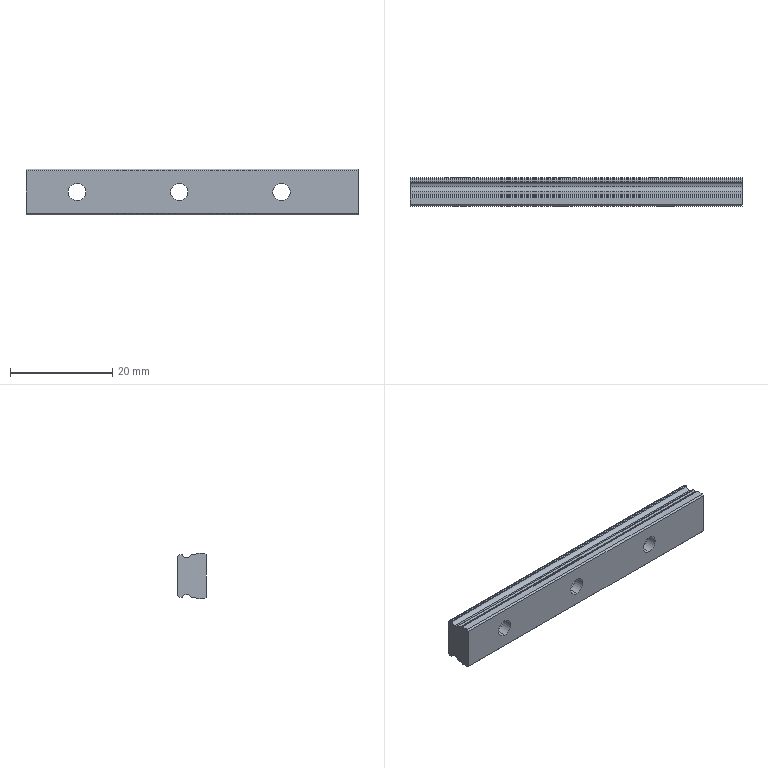Part | SolidWorks | features BaseBody 1, Cut 1, HoleWzd 1, ICE 1, LPattern 1 | 1 solid | 44 faces | box 65 x 5.5 x 9 mm | volume 2567 mm3 | cylinder 25 | plane 19 | commonest cylinder face diameters 0.6 x6 3.4 x6 6.5 x6 0.3 x4 2 x3
STEP:
#1=CARTESIAN_POINT('',(-80.,0.,-1.7));
#2=VERTEX_POINT('',#1);
#3=CARTESIAN_POINT('',(-80.,0.,1.7));
#4=VERTEX_POINT('',#3);
#5=CARTESIAN_POINT('',(-80.,0.,0.));
#6=DIRECTION('',(0.,1.,0.));
#7=DIRECTION('',(0.,0.,1.));
#8=AXIS2_PLACEMENT_3D('',#5,#6,#7);
#9=CIRCLE('',#8,1.7);
#10=EDGE_CURVE('',#2,#4,#9,.T.);
#11=ORIENTED_EDGE('',*,*,#10,.F.);
#12=CARTESIAN_POINT('',(-80.,2.1,-1.7));
#13=VERTEX_POINT('',#12);
#14=CARTESIAN_POINT('',(-80.,5.5,-1.7));
#15=DIRECTION('',(0.,1.,0.));
#16=VECTOR('',#15,1000.);
#17=LINE('',#14,#16);
#18=EDGE_CURVE('',#2,#13,#17,.T.);
#19=ORIENTED_EDGE('',*,*,#18,.T.);
#20=CARTESIAN_POINT('',(-80.,2.1,1.7));
#21=VERTEX_POINT('',#20);
#22=CARTESIAN_POINT('',(-80.,2.1,0.));
#23=DIRECTION('',(0.,1.,0.));
#24=DIRECTION('',(0.,0.,1.));
#25=AXIS2_PLACEMENT_3D('',#22,#23,#24);
#26=CIRCLE('',#25,1.7);
#27=EDGE_CURVE('',#13,#21,#26,.T.);
#28=ORIENTED_EDGE('',*,*,#27,.T.);
#29=CARTESIAN_POINT('',(-80.,5.5,1.7));
#30=DIRECTION('',(0.,1.,0.));
#31=VECTOR('',#30,1000.);
#32=LINE('',#29,#31);
#33=EDGE_CURVE('',#4,#21,#32,.T.);
#34=ORIENTED_EDGE('',*,*,#33,.F.);
#35=EDGE_LOOP('',(#11,#19,#28,#34));
#36=FACE_OUTER_BOUND('',#35,.T.);
#37=CARTESIAN_POINT('',(-80.,5.5,0.));
#38=DIRECTION('',(0.,1.,0.));
#39=DIRECTION('',(0.,0.,1.));
#40=AXIS2_PLACEMENT_3D('',#37,#38,#39);
#41=CYLINDRICAL_SURFACE('',#40,1.7);
#42=ADVANCED_FACE('',(#36),#41,.F.);
#43=CARTESIAN_POINT('',(-80.,2.1,-3.25));
#44=VERTEX_POINT('',#43);
#45=CARTESIAN_POINT('',(-80.,2.1,3.25));
#46=VERTEX_POINT('',#45);
#47=CARTESIAN_POINT('',(-80.,2.1,0.));
#48=DIRECTION('',(0.,1.,0.));
#49=DIRECTION('',(0.,0.,1.));
#50=AXIS2_PLACEMENT_3D('',#47,#48,#49);
#51=CIRCLE('',#50,3.25);
#52=EDGE_CURVE('',#44,#46,#51,.T.);
#53=ORIENTED_EDGE('',*,*,#52,.F.);
#54=CARTESIAN_POINT('',(-80.,5.5,-3.25));
#55=VERTEX_POINT('',#54);
#56=CARTESIAN_POINT('',(-80.,5.5,-3.25));
#57=DIRECTION('',(0.,1.,0.));
#58=VECTOR('',#57,1000.);
#59=LINE('',#56,#58);
#60=EDGE_CURVE('',#44,#55,#59,.T.);
#61=ORIENTED_EDGE('',*,*,#60,.T.);
#62=CARTESIAN_POINT('',(-80.,5.5,3.25));
#63=VERTEX_POINT('',#62);
#64=CARTESIAN_POINT('',(-80.,5.5,0.));
#65=DIRECTION('',(0.,1.,0.));
#66=DIRECTION('',(0.,0.,1.));
#67=AXIS2_PLACEMENT_3D('',#64,#65,#66);
#68=CIRCLE('',#67,3.25);
#69=EDGE_CURVE('',#55,#63,#68,.T.);
#70=ORIENTED_EDGE('',*,*,#69,.T.);
#71=CARTESIAN_POINT('',(-80.,5.5,3.25));
#72=DIRECTION('',(0.,1.,0.));
#73=VECTOR('',#72,1000.);
#74=LINE('',#71,#73);
#75=EDGE_CURVE('',#46,#63,#74,.T.);
#76=ORIENTED_EDGE('',*,*,#75,.F.);
#77=EDGE_LOOP('',(#53,#61,#70,#76));
#78=FACE_OUTER_BOUND('',#77,.T.);
#79=CARTESIAN_POINT('',(-80.,5.5,0.));
#80=DIRECTION('',(0.,1.,0.));
#81=DIRECTION('',(0.,0.,1.));
#82=AXIS2_PLACEMENT_3D('',#79,#80,#81);
#83=CYLINDRICAL_SURFACE('',#82,3.25);
#84=ADVANCED_FACE('',(#78),#83,.F.);
#85=CARTESIAN_POINT('',(-60.,0.,-1.7));
#86=VERTEX_POINT('',#85);
#87=CARTESIAN_POINT('',(-60.,0.,1.7));
#88=VERTEX_POINT('',#87);
#89=CARTESIAN_POINT('',(-60.,0.,0.));
#90=DIRECTION('',(0.,1.,0.));
#91=DIRECTION('',(0.,0.,1.));
#92=AXIS2_PLACEMENT_3D('',#89,#90,#91);
#93=CIRCLE('',#92,1.7);
#94=EDGE_CURVE('',#86,#88,#93,.T.);
#95=ORIENTED_EDGE('',*,*,#94,.F.);
#96=CARTESIAN_POINT('',(-60.,2.1,-1.7));
#97=VERTEX_POINT('',#96);
#98=CARTESIAN_POINT('',(-60.,5.5,-1.7));
#99=DIRECTION('',(0.,1.,0.));
#100=VECTOR('',#99,1000.);
#101=LINE('',#98,#100);
#102=EDGE_CURVE('',#86,#97,#101,.T.);
#103=ORIENTED_EDGE('',*,*,#102,.T.);
#104=CARTESIAN_POINT('',(-60.,2.1,1.7));
#105=VERTEX_POINT('',#104);
#106=CARTESIAN_POINT('',(-60.,2.1,0.));
#107=DIRECTION('',(0.,1.,0.));
#108=DIRECTION('',(0.,0.,1.));
#109=AXIS2_PLACEMENT_3D('',#106,#107,#108);
#110=CIRCLE('',#109,1.7);
#111=EDGE_CURVE('',#97,#105,#110,.T.);
#112=ORIENTED_EDGE('',*,*,#111,.T.);
#113=CARTESIAN_POINT('',(-60.,5.5,1.7));
#114=DIRECTION('',(0.,1.,0.));
#115=VECTOR('',#114,1000.);
#116=LINE('',#113,#115);
#117=EDGE_CURVE('',#88,#105,#116,.T.);
#118=ORIENTED_EDGE('',*,*,#117,.F.);
#119=EDGE_LOOP('',(#95,#103,#112,#118));
#120=FACE_OUTER_BOUND('',#119,.T.);
#121=CARTESIAN_POINT('',(-60.,5.5,0.));
#122=DIRECTION('',(0.,1.,0.));
#123=DIRECTION('',(0.,0.,1.));
#124=AXIS2_PLACEMENT_3D('',#121,#122,#123);
#125=CYLINDRICAL_SURFACE('',#124,1.7);
#126=ADVANCED_FACE('',(#120),#125,.F.);
#127=CARTESIAN_POINT('',(-60.,2.1,-3.25));
#128=VERTEX_POINT('',#127);
#129=CARTESIAN_POINT('',(-60.,2.1,3.25));
#130=VERTEX_POINT('',#129);
#131=CARTESIAN_POINT('',(-60.,2.1,0.));
#132=DIRECTION('',(0.,1.,0.));
#133=DIRECTION('',(0.,0.,1.));
#134=AXIS2_PLACEMENT_3D('',#131,#132,#133);
#135=CIRCLE('',#134,3.25);
#136=EDGE_CURVE('',#128,#130,#135,.T.);
#137=ORIENTED_EDGE('',*,*,#136,.F.);
#138=CARTESIAN_POINT('',(-60.,5.5,-3.25));
#139=VERTEX_POINT('',#138);
#140=CARTESIAN_POINT('',(-60.,5.5,-3.25));
#141=DIRECTION('',(0.,1.,0.));
#142=VECTOR('',#141,1000.);
#143=LINE('',#140,#142);
#144=EDGE_CURVE('',#128,#139,#143,.T.);
#145=ORIENTED_EDGE('',*,*,#144,.T.);
#146=CARTESIAN_POINT('',(-60.,5.5,3.25));
#147=VERTEX_POINT('',#146);
#148=CARTESIAN_POINT('',(-60.,5.5,0.));
#149=DIRECTION('',(0.,1.,0.));
#150=DIRECTION('',(0.,0.,1.));
#151=AXIS2_PLACEMENT_3D('',#148,#149,#150);
#152=CIRCLE('',#151,3.25);
#153=EDGE_CURVE('',#139,#147,#152,.T.);
#154=ORIENTED_EDGE('',*,*,#153,.T.);
#155=CARTESIAN_POINT('',(-60.,5.5,3.25));
#156=DIRECTION('',(0.,1.,0.));
#157=VECTOR('',#156,1000.);
#158=LINE('',#155,#157);
#159=EDGE_CURVE('',#130,#147,#158,.T.);
#160=ORIENTED_EDGE('',*,*,#159,.F.);
#161=EDGE_LOOP('',(#137,#145,#154,#160));
#162=FACE_OUTER_BOUND('',#161,.T.);
#163=CARTESIAN_POINT('',(-60.,5.5,0.));
#164=DIRECTION('',(0.,1.,0.));
#165=DIRECTION('',(0.,0.,1.));
#166=AXIS2_PLACEMENT_3D('',#163,#164,#165);
#167=CYLINDRICAL_SURFACE('',#166,3.25);
#168=ADVANCED_FACE('',(#162),#167,.F.);
#169=CARTESIAN_POINT('',(-40.,2.1,-3.25));
#170=VERTEX_POINT('',#169);
#171=CARTESIAN_POINT('',(-40.,2.1,3.25));
#172=VERTEX_POINT('',#171);
#173=CARTESIAN_POINT('',(-40.,2.1,0.));
#174=DIRECTION('',(0.,1.,0.));
#175=DIRECTION('',(0.,0.,1.));
#176=AXIS2_PLACEMENT_3D('',#173,#174,#175);
#177=CIRCLE('',#176,3.25);
#178=EDGE_CURVE('',#170,#172,#177,.T.);
#179=ORIENTED_EDGE('',*,*,#178,.F.);
#180=CARTESIAN_POINT('',(-40.,5.5,-3.25));
#181=VERTEX_POINT('',#180);
#182=CARTESIAN_POINT('',(-40.,5.5,-3.25));
#183=DIRECTION('',(0.,1.,0.));
#184=VECTOR('',#183,1000.);
#185=LINE('',#182,#184);
#186=EDGE_CURVE('',#170,#181,#185,.T.);
#187=ORIENTED_EDGE('',*,*,#186,.T.);
#188=CARTESIAN_POINT('',(-40.,5.5,3.25));
#189=VERTEX_POINT('',#188);
#190=CARTESIAN_POINT('',(-40.,5.5,0.));
#191=DIRECTION('',(0.,1.,0.));
#192=DIRECTION('',(0.,0.,1.));
#193=AXIS2_PLACEMENT_3D('',#190,#191,#192);
#194=CIRCLE('',#193,3.25);
#195=EDGE_CURVE('',#181,#189,#194,.T.);
#196=ORIENTED_EDGE('',*,*,#195,.T.);
#197=CARTESIAN_POINT('',(-40.,5.5,3.25));
#198=DIRECTION('',(0.,1.,0.));
#199=VECTOR('',#198,1000.);
#200=LINE('',#197,#199);
#201=EDGE_CURVE('',#172,#189,#200,.T.);
#202=ORIENTED_EDGE('',*,*,#201,.F.);
#203=EDGE_LOOP('',(#179,#187,#196,#202));
#204=FACE_OUTER_BOUND('',#203,.T.);
#205=CARTESIAN_POINT('',(-40.,5.5,0.));
#206=DIRECTION('',(0.,1.,0.));
#207=DIRECTION('',(0.,0.,1.));
#208=AXIS2_PLACEMENT_3D('',#205,#206,#207);
#209=CYLINDRICAL_SURFACE('',#208,3.25);
#210=ADVANCED_FACE('',(#204),#209,.F.);
#211=CARTESIAN_POINT('',(-40.,0.,-1.7));
#212=VERTEX_POINT('',#211);
#213=CARTESIAN_POINT('',(-40.,0.,1.7));
#214=VERTEX_POINT('',#213);
#215=CARTESIAN_POINT('',(-40.,0.,0.));
#216=DIRECTION('',(0.,1.,0.));
#217=DIRECTION('',(0.,0.,1.));
#218=AXIS2_PLACEMENT_3D('',#215,#216,#217);
#219=CIRCLE('',#218,1.7);
#220=EDGE_CURVE('',#212,#214,#219,.T.);
#221=ORIENTED_EDGE('',*,*,#220,.F.);
#222=CARTESIAN_POINT('',(-40.,2.1,-1.7));
#223=VERTEX_POINT('',#222);
#224=CARTESIAN_POINT('',(-40.,5.5,-1.7));
#225=DIRECTION('',(0.,1.,0.));
#226=VECTOR('',#225,1000.);
#227=LINE('',#224,#226);
#228=EDGE_CURVE('',#212,#223,#227,.T.);
#229=ORIENTED_EDGE('',*,*,#228,.T.);
#230=CARTESIAN_POINT('',(-40.,2.1,1.7));
#231=VERTEX_POINT('',#230);
#232=CARTESIAN_POINT('',(-40.,2.1,0.));
#233=DIRECTION('',(0.,1.,0.));
#234=DIRECTION('',(0.,0.,1.));
#235=AXIS2_PLACEMENT_3D('',#232,#233,#234);
#236=CIRCLE('',#235,1.7);
#237=EDGE_CURVE('',#223,#231,#236,.T.);
#238=ORIENTED_EDGE('',*,*,#237,.T.);
#239=CARTESIAN_POINT('',(-40.,5.5,1.7));
#240=DIRECTION('',(0.,1.,0.));
#241=VECTOR('',#240,1000.);
#242=LINE('',#239,#241);
#243=EDGE_CURVE('',#214,#231,#242,.T.);
#244=ORIENTED_EDGE('',*,*,#243,.F.);
#245=EDGE_LOOP('',(#221,#229,#238,#244));
#246=FACE_OUTER_BOUND('',#245,.T.);
#247=CARTESIAN_POINT('',(-40.,5.5,0.));
#248=DIRECTION('',(0.,1.,0.));
#249=DIRECTION('',(0.,0.,1.));
#250=AXIS2_PLACEMENT_3D('',#247,#248,#249);
#251=CYLINDRICAL_SURFACE('',#250,1.7);
#252=ADVANCED_FACE('',(#246),#251,.F.);
#253=CARTESIAN_POINT('',(-90.,3.8,3.6));
#254=VERTEX_POINT('',#253);
#255=CARTESIAN_POINT('',(-90.,4.678,4.122));
#256=VERTEX_POINT('',#255);
#257=CARTESIAN_POINT('',(-90.,3.8,4.6));
#258=DIRECTION('',(1.,0.,0.));
#259=DIRECTION('',(0.,0.,1.));
#260=AXIS2_PLACEMENT_3D('',#257,#258,#259);
#261=CIRCLE('',#260,1.);
#262=EDGE_CURVE('',#254,#256,#261,.T.);
#263=ORIENTED_EDGE('',*,*,#262,.F.);
#264=CARTESIAN_POINT('',(-25.,3.8,3.6));
#265=VERTEX_POINT('',#264);
#266=CARTESIAN_POINT('',(30.,3.8,3.6));
#267=DIRECTION('',(1.,0.,0.));
#268=VECTOR('',#267,1000.);
#269=LINE('',#266,#268);
#270=EDGE_CURVE('',#254,#265,#269,.T.);
#271=ORIENTED_EDGE('',*,*,#270,.T.);
#272=CARTESIAN_POINT('',(-25.,4.678,4.122));
#273=VERTEX_POINT('',#272);
#274=CARTESIAN_POINT('',(-25.,3.8,4.6));
#275=DIRECTION('',(-1.,0.,0.));
#276=DIRECTION('',(0.,0.,-1.));
#277=AXIS2_PLACEMENT_3D('',#274,#275,#276);
#278=CIRCLE('',#277,1.);
#279=EDGE_CURVE('',#273,#265,#278,.T.);
#280=ORIENTED_EDGE('',*,*,#279,.F.);
#281=CARTESIAN_POINT('',(30.,4.678,4.122));
#282=DIRECTION('',(1.,0.,0.));
#283=VECTOR('',#282,1000.);
#284=LINE('',#281,#283);
#285=EDGE_CURVE('',#256,#273,#284,.T.);
#286=ORIENTED_EDGE('',*,*,#285,.F.);
#287=EDGE_LOOP('',(#263,#271,#280,#286));
#288=FACE_OUTER_BOUND('',#287,.T.);
#289=CARTESIAN_POINT('',(30.,3.8,4.6));
#290=DIRECTION('',(1.,0.,0.));
#291=DIRECTION('',(0.,0.,-1.));
#292=AXIS2_PLACEMENT_3D('',#289,#290,#291);
#293=CYLINDRICAL_SURFACE('',#292,1.);
#294=ADVANCED_FACE('',(#288),#293,.F.);
#295=CARTESIAN_POINT('',(-25.,2.02,-4.26));
#296=VERTEX_POINT('',#295);
#297=CARTESIAN_POINT('',(-25.,2.2,-4.2));
#298=VERTEX_POINT('',#297);
#299=CARTESIAN_POINT('',(-25.,2.2,-4.5));
#300=DIRECTION('',(-1.,0.,0.));
#301=DIRECTION('',(0.,0.,-1.));
#302=AXIS2_PLACEMENT_3D('',#299,#300,#301);
#303=CIRCLE('',#302,0.3);
#304=EDGE_CURVE('',#296,#298,#303,.T.);
#305=ORIENTED_EDGE('',*,*,#304,.F.);
#306=CARTESIAN_POINT('',(-90.,2.02,-4.26));
#307=VERTEX_POINT('',#306);
#308=CARTESIAN_POINT('',(30.,2.02,-4.26));
#309=DIRECTION('',(-1.,0.,0.));
#310=VECTOR('',#309,1000.);
#311=LINE('',#308,#310);
#312=EDGE_CURVE('',#296,#307,#311,.T.);
#313=ORIENTED_EDGE('',*,*,#312,.T.);
#314=CARTESIAN_POINT('',(-90.,2.2,-4.2));
#315=VERTEX_POINT('',#314);
#316=CARTESIAN_POINT('',(-90.,2.2,-4.5));
#317=DIRECTION('',(1.,0.,0.));
#318=DIRECTION('',(0.,0.,1.));
#319=AXIS2_PLACEMENT_3D('',#316,#317,#318);
#320=CIRCLE('',#319,0.3);
#321=EDGE_CURVE('',#315,#307,#320,.T.);
#322=ORIENTED_EDGE('',*,*,#321,.F.);
#323=CARTESIAN_POINT('',(30.,2.2,-4.2));
#324=DIRECTION('',(1.,0.,0.));
#325=VECTOR('',#324,1000.);
#326=LINE('',#323,#325);
#327=EDGE_CURVE('',#315,#298,#326,.T.);
#328=ORIENTED_EDGE('',*,*,#327,.T.);
#329=EDGE_LOOP('',(#305,#313,#322,#328));
#330=FACE_OUTER_BOUND('',#329,.T.);
#331=CARTESIAN_POINT('',(30.,2.2,-4.5));
#332=DIRECTION('',(1.,0.,0.));
#333=DIRECTION('',(0.,0.,-1.));
#334=AXIS2_PLACEMENT_3D('',#331,#332,#333);
#335=CYLINDRICAL_SURFACE('',#334,0.3);
#336=ADVANCED_FACE('',(#330),#335,.F.);
#337=CARTESIAN_POINT('',(-25.,2.2,4.2));
#338=VERTEX_POINT('',#337);
#339=CARTESIAN_POINT('',(-25.,2.02,4.26));
#340=VERTEX_POINT('',#339);
#341=CARTESIAN_POINT('',(-25.,2.2,4.5));
#342=DIRECTION('',(-1.,0.,0.));
#343=DIRECTION('',(0.,0.,-1.));
#344=AXIS2_PLACEMENT_3D('',#341,#342,#343);
#345=CIRCLE('',#344,0.3);
#346=EDGE_CURVE('',#338,#340,#345,.T.);
#347=ORIENTED_EDGE('',*,*,#346,.F.);
#348=CARTESIAN_POINT('',(-90.,2.2,4.2));
#349=VERTEX_POINT('',#348);
#350=CARTESIAN_POINT('',(30.,2.2,4.2));
#351=DIRECTION('',(-1.,0.,0.));
#352=VECTOR('',#351,1000.);
#353=LINE('',#350,#352);
#354=EDGE_CURVE('',#338,#349,#353,.T.);
#355=ORIENTED_EDGE('',*,*,#354,.T.);
#356=CARTESIAN_POINT('',(-90.,2.02,4.26));
#357=VERTEX_POINT('',#356);
#358=CARTESIAN_POINT('',(-90.,2.2,4.5));
#359=DIRECTION('',(1.,0.,0.));
#360=DIRECTION('',(0.,0.,1.));
#361=AXIS2_PLACEMENT_3D('',#358,#359,#360);
#362=CIRCLE('',#361,0.3);
#363=EDGE_CURVE('',#357,#349,#362,.T.);
#364=ORIENTED_EDGE('',*,*,#363,.F.);
#365=CARTESIAN_POINT('',(30.,2.02,4.26));
#366=DIRECTION('',(1.,0.,0.));
#367=VECTOR('',#366,1000.);
#368=LINE('',#365,#367);
#369=EDGE_CURVE('',#357,#340,#368,.T.);
#370=ORIENTED_EDGE('',*,*,#369,.T.);
#371=EDGE_LOOP('',(#347,#355,#364,#370));
#372=FACE_OUTER_BOUND('',#371,.T.);
#373=CARTESIAN_POINT('',(30.,2.2,4.5));
#374=DIRECTION('',(1.,0.,0.));
#375=DIRECTION('',(0.,0.,-1.));
#376=AXIS2_PLACEMENT_3D('',#373,#374,#375);
#377=CYLINDRICAL_SURFACE('',#376,0.3);
#378=ADVANCED_FACE('',(#372),#377,.F.);
#379=CARTESIAN_POINT('',(-25.,1.78,4.44));
#380=VERTEX_POINT('',#379);
#381=CARTESIAN_POINT('',(-25.,2.02,4.26));
#382=DIRECTION('',(0.,-0.8,0.6));
#383=VECTOR('',#382,1000.);
#384=LINE('',#381,#383);
#385=EDGE_CURVE('',#340,#380,#384,.T.);
#386=ORIENTED_EDGE('',*,*,#385,.F.);
#387=ORIENTED_EDGE('',*,*,#369,.F.);
#388=CARTESIAN_POINT('',(-90.,1.78,4.44));
#389=VERTEX_POINT('',#388);
#390=CARTESIAN_POINT('',(-90.,1.78,4.44));
#391=DIRECTION('',(0.,0.8,-0.6));
#392=VECTOR('',#391,1000.);
#393=LINE('',#390,#392);
#394=EDGE_CURVE('',#389,#357,#393,.T.);
#395=ORIENTED_EDGE('',*,*,#394,.F.);
#396=CARTESIAN_POINT('',(30.,1.78,4.44));
#397=DIRECTION('',(-1.,0.,0.));
#398=VECTOR('',#397,1000.);
#399=LINE('',#396,#398);
#400=EDGE_CURVE('',#380,#389,#399,.T.);
#401=ORIENTED_EDGE('',*,*,#400,.F.);
#402=EDGE_LOOP('',(#386,#387,#395,#401));
#403=FACE_OUTER_BOUND('',#402,.T.);
#404=CARTESIAN_POINT('',(30.,2.02,4.26));
#405=DIRECTION('',(0.,-0.6,-0.8));
#406=DIRECTION('',(0.,0.8,-0.6));
#407=AXIS2_PLACEMENT_3D('',#404,#405,#406);
#408=PLANE('',#407);
#409=ADVANCED_FACE('',(#403),#408,.F.);
#410=CARTESIAN_POINT('',(-25.,1.78,-4.44));
#411=VERTEX_POINT('',#410);
#412=CARTESIAN_POINT('',(-25.,1.78,-4.44));
#413=DIRECTION('',(0.,0.8,0.6));
#414=VECTOR('',#413,1000.);
#415=LINE('',#412,#414);
#416=EDGE_CURVE('',#411,#296,#415,.T.);
#417=ORIENTED_EDGE('',*,*,#416,.F.);
#418=CARTESIAN_POINT('',(-90.,1.78,-4.44));
#419=VERTEX_POINT('',#418);
#420=CARTESIAN_POINT('',(30.,1.78,-4.44));
#421=DIRECTION('',(1.,0.,0.));
#422=VECTOR('',#421,1000.);
#423=LINE('',#420,#422);
#424=EDGE_CURVE('',#419,#411,#423,.T.);
#425=ORIENTED_EDGE('',*,*,#424,.F.);
#426=CARTESIAN_POINT('',(-90.,2.02,-4.26));
#427=DIRECTION('',(0.,-0.8,-0.6));
#428=VECTOR('',#427,1000.);
#429=LINE('',#426,#428);
#430=EDGE_CURVE('',#307,#419,#429,.T.);
#431=ORIENTED_EDGE('',*,*,#430,.F.);
#432=ORIENTED_EDGE('',*,*,#312,.F.);
#433=EDGE_LOOP('',(#417,#425,#431,#432));
#434=FACE_OUTER_BOUND('',#433,.T.);
#435=CARTESIAN_POINT('',(30.,1.78,-4.44));
#436=DIRECTION('',(0.,-0.6,0.8));
#437=DIRECTION('',(0.,-0.8,-0.6));
#438=AXIS2_PLACEMENT_3D('',#435,#436,#437);
#439=PLANE('',#438);
#440=ADVANCED_FACE('',(#434),#439,.F.);
#441=CARTESIAN_POINT('',(-25.,2.79,-4.2));
#442=VERTEX_POINT('',#441);
#443=CARTESIAN_POINT('',(-25.,2.2,-4.2));
#444=DIRECTION('',(0.,1.,0.));
#445=VECTOR('',#444,1000.);
#446=LINE('',#443,#445);
#447=EDGE_CURVE('',#298,#442,#446,.T.);
#448=ORIENTED_EDGE('',*,*,#447,.F.);
#449=ORIENTED_EDGE('',*,*,#327,.F.);
#450=CARTESIAN_POINT('',(-90.,2.79,-4.2));
#451=VERTEX_POINT('',#450);
#452=CARTESIAN_POINT('',(-90.,2.79,-4.2));
#453=DIRECTION('',(0.,-1.,0.));
#454=VECTOR('',#453,1000.);
#455=LINE('',#452,#454);
#456=EDGE_CURVE('',#451,#315,#455,.T.);
#457=ORIENTED_EDGE('',*,*,#456,.F.);
#458=CARTESIAN_POINT('',(30.,2.79,-4.2));
#459=DIRECTION('',(-1.,0.,0.));
#460=VECTOR('',#459,1000.);
#461=LINE('',#458,#460);
#462=EDGE_CURVE('',#442,#451,#461,.T.);
#463=ORIENTED_EDGE('',*,*,#462,.F.);
#464=EDGE_LOOP('',(#448,#449,#457,#463));
#465=FACE_OUTER_BOUND('',#464,.T.);
#466=CARTESIAN_POINT('',(30.,2.2,-4.2));
#467=DIRECTION('',(0.,0.,1.));
#468=DIRECTION('',(1.,0.,0.));
#469=AXIS2_PLACEMENT_3D('',#466,#467,#468);
#470=PLANE('',#469);
#471=ADVANCED_FACE('',(#465),#470,.F.);
#472=CARTESIAN_POINT('',(-25.,4.81,-4.2));
#473=VERTEX_POINT('',#472);
#474=CARTESIAN_POINT('',(-25.,5.1,-4.2));
#475=VERTEX_POINT('',#474);
#476=CARTESIAN_POINT('',(-25.,4.81,-4.2));
#477=DIRECTION('',(0.,1.,0.));
#478=VECTOR('',#477,1000.);
#479=LINE('',#476,#478);
#480=EDGE_CURVE('',#473,#475,#479,.T.);
#481=ORIENTED_EDGE('',*,*,#480,.F.);
#482=CARTESIAN_POINT('',(-90.,4.81,-4.2));
#483=VERTEX_POINT('',#482);
#484=CARTESIAN_POINT('',(30.,4.81,-4.2));
#485=DIRECTION('',(1.,0.,0.));
#486=VECTOR('',#485,1000.);
#487=LINE('',#484,#486);
#488=EDGE_CURVE('',#483,#473,#487,.T.);
#489=ORIENTED_EDGE('',*,*,#488,.F.);
#490=CARTESIAN_POINT('',(-90.,5.1,-4.2));
#491=VERTEX_POINT('',#490);
#492=CARTESIAN_POINT('',(-90.,5.1,-4.2));
#493=DIRECTION('',(0.,-1.,0.));
#494=VECTOR('',#493,1000.);
#495=LINE('',#492,#494);
#496=EDGE_CURVE('',#491,#483,#495,.T.);
#497=ORIENTED_EDGE('',*,*,#496,.F.);
#498=CARTESIAN_POINT('',(30.,5.1,-4.2));
#499=DIRECTION('',(-1.,0.,0.));
#500=VECTOR('',#499,1000.);
#501=LINE('',#498,#500);
#502=EDGE_CURVE('',#475,#491,#501,.T.);
#503=ORIENTED_EDGE('',*,*,#502,.F.);
#504=EDGE_LOOP('',(#481,#489,#497,#503));
#505=FACE_OUTER_BOUND('',#504,.T.);
#506=CARTESIAN_POINT('',(30.,4.81,-4.2));
#507=DIRECTION('',(0.,0.,1.));
#508=DIRECTION('',(1.,0.,0.));
#509=AXIS2_PLACEMENT_3D('',#506,#507,#508);
#510=PLANE('',#509);
#511=ADVANCED_FACE('',(#505),#510,.F.);
#512=CARTESIAN_POINT('',(-90.,5.325,-4.098));
#513=VERTEX_POINT('',#512);
#514=CARTESIAN_POINT('',(-25.,5.325,-4.098));
#515=VERTEX_POINT('',#514);
#516=CARTESIAN_POINT('',(30.,5.325,-4.098));
#517=DIRECTION('',(1.,0.,0.));
#518=VECTOR('',#517,1000.);
#519=LINE('',#516,#518);
#520=EDGE_CURVE('',#513,#515,#519,.T.);
#521=ORIENTED_EDGE('',*,*,#520,.T.);
#522=CARTESIAN_POINT('',(-25.,5.1,-3.9));
#523=DIRECTION('',(1.,0.,0.));
#524=DIRECTION('',(0.,0.,-1.));
#525=AXIS2_PLACEMENT_3D('',#522,#523,#524);
#526=CIRCLE('',#525,0.3);
#527=EDGE_CURVE('',#475,#515,#526,.T.);
#528=ORIENTED_EDGE('',*,*,#527,.F.);
#529=ORIENTED_EDGE('',*,*,#502,.T.);
#530=CARTESIAN_POINT('',(-90.,5.1,-3.9));
#531=DIRECTION('',(-1.,0.,0.));
#532=DIRECTION('',(0.,0.,1.));
#533=AXIS2_PLACEMENT_3D('',#530,#531,#532);
#534=CIRCLE('',#533,0.3);
#535=EDGE_CURVE('',#513,#491,#534,.T.);
#536=ORIENTED_EDGE('',*,*,#535,.F.);
#537=EDGE_LOOP('',(#521,#528,#529,#536));
#538=FACE_OUTER_BOUND('',#537,.T.);
#539=CARTESIAN_POINT('',(30.,5.1,-3.9));
#540=DIRECTION('',(1.,0.,0.));
#541=DIRECTION('',(0.,0.,-1.));
#542=AXIS2_PLACEMENT_3D('',#539,#540,#541);
#543=CYLINDRICAL_SURFACE('',#542,0.3);
#544=ADVANCED_FACE('',(#538),#543,.T.);
#545=CARTESIAN_POINT('',(-90.,5.1,4.2));
#546=VERTEX_POINT('',#545);
#547=CARTESIAN_POINT('',(-25.,5.1,4.2));
#548=VERTEX_POINT('',#547);
#549=CARTESIAN_POINT('',(30.,5.1,4.2));
#550=DIRECTION('',(1.,0.,0.));
#551=VECTOR('',#550,1000.);
#552=LINE('',#549,#551);
#553=EDGE_CURVE('',#546,#548,#552,.T.);
#554=ORIENTED_EDGE('',*,*,#553,.T.);
#555=CARTESIAN_POINT('',(-25.,5.325,4.098));
#556=VERTEX_POINT('',#555);
#557=CARTESIAN_POINT('',(-25.,5.1,3.9));
#558=DIRECTION('',(1.,0.,0.));
#559=DIRECTION('',(0.,0.,-1.));
#560=AXIS2_PLACEMENT_3D('',#557,#558,#559);
#561=CIRCLE('',#560,0.3);
#562=EDGE_CURVE('',#556,#548,#561,.T.);
#563=ORIENTED_EDGE('',*,*,#562,.F.);
#564=CARTESIAN_POINT('',(-90.,5.325,4.098));
#565=VERTEX_POINT('',#564);
#566=CARTESIAN_POINT('',(30.,5.325,4.098));
#567=DIRECTION('',(-1.,0.,0.));
#568=VECTOR('',#567,1000.);
#569=LINE('',#566,#568);
#570=EDGE_CURVE('',#556,#565,#569,.T.);
#571=ORIENTED_EDGE('',*,*,#570,.T.);
#572=CARTESIAN_POINT('',(-90.,5.1,3.9));
#573=DIRECTION('',(-1.,0.,0.));
#574=DIRECTION('',(0.,0.,1.));
#575=AXIS2_PLACEMENT_3D('',#572,#573,#574);
#576=CIRCLE('',#575,0.3);
#577=EDGE_CURVE('',#546,#565,#576,.T.);
#578=ORIENTED_EDGE('',*,*,#577,.F.);
#579=EDGE_LOOP('',(#554,#563,#571,#578));
#580=FACE_OUTER_BOUND('',#579,.T.);
#581=CARTESIAN_POINT('',(30.,5.1,3.9));
#582=DIRECTION('',(1.,0.,0.));
#583=DIRECTION('',(0.,0.,-1.));
#584=AXIS2_PLACEMENT_3D('',#581,#582,#583);
#585=CYLINDRICAL_SURFACE('',#584,0.3);
#586=ADVANCED_FACE('',(#580),#585,.T.);
#587=CARTESIAN_POINT('',(-25.,4.81,4.2));
#588=VERTEX_POINT('',#587);
#589=CARTESIAN_POINT('',(-25.,5.1,4.2));
#590=DIRECTION('',(0.,-1.,0.));
#591=VECTOR('',#590,1000.);
#592=LINE('',#589,#591);
#593=EDGE_CURVE('',#548,#588,#592,.T.);
#594=ORIENTED_EDGE('',*,*,#593,.F.);
#595=ORIENTED_EDGE('',*,*,#553,.F.);
#596=CARTESIAN_POINT('',(-90.,4.81,4.2));
#597=VERTEX_POINT('',#596);
#598=CARTESIAN_POINT('',(-90.,4.81,4.2));
#599=DIRECTION('',(0.,1.,0.));
#600=VECTOR('',#599,1000.);
#601=LINE('',#598,#600);
#602=EDGE_CURVE('',#597,#546,#601,.T.);
#603=ORIENTED_EDGE('',*,*,#602,.F.);
#604=CARTESIAN_POINT('',(30.,4.81,4.2));
#605=DIRECTION('',(-1.,0.,0.));
#606=VECTOR('',#605,1000.);
#607=LINE('',#604,#606);
#608=EDGE_CURVE('',#588,#597,#607,.T.);
#609=ORIENTED_EDGE('',*,*,#608,.F.);
#610=EDGE_LOOP('',(#594,#595,#603,#609));
#611=FACE_OUTER_BOUND('',#610,.T.);
#612=CARTESIAN_POINT('',(30.,5.1,4.2));
#613=DIRECTION('',(0.,0.,-1.));
#614=DIRECTION('',(-1.,0.,0.));
#615=AXIS2_PLACEMENT_3D('',#612,#613,#614);
#616=PLANE('',#615);
#617=ADVANCED_FACE('',(#611),#616,.F.);
#618=CARTESIAN_POINT('',(-25.,2.79,4.2));
#619=VERTEX_POINT('',#618);
#620=CARTESIAN_POINT('',(-25.,2.79,4.2));
#621=DIRECTION('',(0.,-1.,0.));
#622=VECTOR('',#621,1000.);
#623=LINE('',#620,#622);
#624=EDGE_CURVE('',#619,#338,#623,.T.);
#625=ORIENTED_EDGE('',*,*,#624,.F.);
#626=CARTESIAN_POINT('',(-90.,2.79,4.2));
#627=VERTEX_POINT('',#626);
#628=CARTESIAN_POINT('',(30.,2.79,4.2));
#629=DIRECTION('',(1.,0.,0.));
#630=VECTOR('',#629,1000.);
#631=LINE('',#628,#630);
#632=EDGE_CURVE('',#627,#619,#631,.T.);
#633=ORIENTED_EDGE('',*,*,#632,.F.);
#634=CARTESIAN_POINT('',(-90.,2.2,4.2));
#635=DIRECTION('',(0.,1.,0.));
#636=VECTOR('',#635,1000.);
#637=LINE('',#634,#636);
#638=EDGE_CURVE('',#349,#627,#637,.T.);
#639=ORIENTED_EDGE('',*,*,#638,.F.);
#640=ORIENTED_EDGE('',*,*,#354,.F.);
#641=EDGE_LOOP('',(#625,#633,#639,#640));
#642=FACE_OUTER_BOUND('',#641,.T.);
#643=CARTESIAN_POINT('',(30.,2.79,4.2));
#644=DIRECTION('',(0.,0.,-1.));
#645=DIRECTION('',(-1.,0.,0.));
#646=AXIS2_PLACEMENT_3D('',#643,#644,#645);
#647=PLANE('',#646);
#648=ADVANCED_FACE('',(#642),#647,.F.);
#649=CARTESIAN_POINT('',(-90.,1.6,4.5));
#650=VERTEX_POINT('',#649);
#651=CARTESIAN_POINT('',(-25.,1.6,4.5));
#652=VERTEX_POINT('',#651);
#653=CARTESIAN_POINT('',(30.,1.6,4.5));
#654=DIRECTION('',(1.,0.,0.));
#655=VECTOR('',#654,1000.);
#656=LINE('',#653,#655);
#657=EDGE_CURVE('',#650,#652,#656,.T.);
#658=ORIENTED_EDGE('',*,*,#657,.T.);
#659=CARTESIAN_POINT('',(-25.,1.6,4.2));
#660=DIRECTION('',(1.,0.,0.));
#661=DIRECTION('',(0.,0.,-1.));
#662=AXIS2_PLACEMENT_3D('',#659,#660,#661);
#663=CIRCLE('',#662,0.3);
#664=EDGE_CURVE('',#380,#652,#663,.T.);
#665=ORIENTED_EDGE('',*,*,#664,.F.);
#666=ORIENTED_EDGE('',*,*,#400,.T.);
#667=CARTESIAN_POINT('',(-90.,1.6,4.2));
#668=DIRECTION('',(-1.,0.,0.));
#669=DIRECTION('',(0.,0.,1.));
#670=AXIS2_PLACEMENT_3D('',#667,#668,#669);
#671=CIRCLE('',#670,0.3);
#672=EDGE_CURVE('',#650,#389,#671,.T.);
#673=ORIENTED_EDGE('',*,*,#672,.F.);
#674=EDGE_LOOP('',(#658,#665,#666,#673));
#675=FACE_OUTER_BOUND('',#674,.T.);
#676=CARTESIAN_POINT('',(30.,1.6,4.2));
#677=DIRECTION('',(1.,0.,0.));
#678=DIRECTION('',(0.,0.,-1.));
#679=AXIS2_PLACEMENT_3D('',#676,#677,#678);
#680=CYLINDRICAL_SURFACE('',#679,0.3);
#681=ADVANCED_FACE('',(#675),#680,.T.);
#682=ORIENTED_EDGE('',*,*,#424,.T.);
#683=CARTESIAN_POINT('',(-25.,1.6,-4.5));
#684=VERTEX_POINT('',#683);
#685=CARTESIAN_POINT('',(-25.,1.6,-4.2));
#686=DIRECTION('',(1.,0.,0.));
#687=DIRECTION('',(0.,0.,-1.));
#688=AXIS2_PLACEMENT_3D('',#685,#686,#687);
#689=CIRCLE('',#688,0.3);
#690=EDGE_CURVE('',#684,#411,#689,.T.);
#691=ORIENTED_EDGE('',*,*,#690,.F.);
#692=CARTESIAN_POINT('',(-90.,1.6,-4.5));
#693=VERTEX_POINT('',#692);
#694=CARTESIAN_POINT('',(30.,1.6,-4.5));
#695=DIRECTION('',(-1.,0.,0.));
#696=VECTOR('',#695,1000.);
#697=LINE('',#694,#696);
#698=EDGE_CURVE('',#684,#693,#697,.T.);
#699=ORIENTED_EDGE('',*,*,#698,.T.);
#700=CARTESIAN_POINT('',(-90.,1.6,-4.2));
#701=DIRECTION('',(-1.,0.,0.));
#702=DIRECTION('',(0.,0.,1.));
#703=AXIS2_PLACEMENT_3D('',#700,#701,#702);
#704=CIRCLE('',#703,0.3);
#705=EDGE_CURVE('',#419,#693,#704,.T.);
#706=ORIENTED_EDGE('',*,*,#705,.F.);
#707=EDGE_LOOP('',(#682,#691,#699,#706));
#708=FACE_OUTER_BOUND('',#707,.T.);
#709=CARTESIAN_POINT('',(30.,1.6,-4.2));
#710=DIRECTION('',(1.,0.,0.));
#711=DIRECTION('',(0.,0.,-1.));
#712=AXIS2_PLACEMENT_3D('',#709,#710,#711);
#713=CYLINDRICAL_SURFACE('',#712,0.3);
#714=ADVANCED_FACE('',(#708),#713,.T.);
#715=CARTESIAN_POINT('',(-90.,2.922,-4.122));
#716=VERTEX_POINT('',#715);
#717=CARTESIAN_POINT('',(-25.,2.922,-4.122));
#718=VERTEX_POINT('',#717);
#719=CARTESIAN_POINT('',(30.,2.922,-4.122));
#720=DIRECTION('',(1.,0.,0.));
#721=VECTOR('',#720,1000.);
#722=LINE('',#719,#721);
#723=EDGE_CURVE('',#716,#718,#722,.T.);
#724=ORIENTED_EDGE('',*,*,#723,.T.);
#725=CARTESIAN_POINT('',(-25.,2.79,-4.05));
#726=DIRECTION('',(1.,0.,0.));
#727=DIRECTION('',(0.,0.,-1.));
#728=AXIS2_PLACEMENT_3D('',#725,#726,#727);
#729=CIRCLE('',#728,0.15);
#730=EDGE_CURVE('',#442,#718,#729,.T.);
#731=ORIENTED_EDGE('',*,*,#730,.F.);
#732=ORIENTED_EDGE('',*,*,#462,.T.);
#733=CARTESIAN_POINT('',(-90.,2.79,-4.05));
#734=DIRECTION('',(-1.,0.,0.));
#735=DIRECTION('',(0.,0.,1.));
#736=AXIS2_PLACEMENT_3D('',#733,#734,#735);
#737=CIRCLE('',#736,0.15);
#738=EDGE_CURVE('',#716,#451,#737,.T.);
#739=ORIENTED_EDGE('',*,*,#738,.F.);
#740=EDGE_LOOP('',(#724,#731,#732,#739));
#741=FACE_OUTER_BOUND('',#740,.T.);
#742=CARTESIAN_POINT('',(30.,2.79,-4.05));
#743=DIRECTION('',(1.,0.,0.));
#744=DIRECTION('',(0.,0.,-1.));
#745=AXIS2_PLACEMENT_3D('',#742,#743,#744);
#746=CYLINDRICAL_SURFACE('',#745,0.15);
#747=ADVANCED_FACE('',(#741),#746,.T.);
#748=ORIENTED_EDGE('',*,*,#488,.T.);
#749=CARTESIAN_POINT('',(-25.,4.678,-4.122));
#750=VERTEX_POINT('',#749);
#751=CARTESIAN_POINT('',(-25.,4.81,-4.05));
#752=DIRECTION('',(1.,0.,0.));
#753=DIRECTION('',(0.,0.,-1.));
#754=AXIS2_PLACEMENT_3D('',#751,#752,#753);
#755=CIRCLE('',#754,0.15);
#756=EDGE_CURVE('',#750,#473,#755,.T.);
#757=ORIENTED_EDGE('',*,*,#756,.F.);
#758=CARTESIAN_POINT('',(-90.,4.678,-4.122));
#759=VERTEX_POINT('',#758);
#760=CARTESIAN_POINT('',(30.,4.678,-4.122));
#761=DIRECTION('',(-1.,0.,0.));
#762=VECTOR('',#761,1000.);
#763=LINE('',#760,#762);
#764=EDGE_CURVE('',#750,#759,#763,.T.);
#765=ORIENTED_EDGE('',*,*,#764,.T.);
#766=CARTESIAN_POINT('',(-90.,4.81,-4.05));
#767=DIRECTION('',(-1.,0.,0.));
#768=DIRECTION('',(0.,0.,1.));
#769=AXIS2_PLACEMENT_3D('',#766,#767,#768);
#770=CIRCLE('',#769,0.15);
#771=EDGE_CURVE('',#483,#759,#770,.T.);
#772=ORIENTED_EDGE('',*,*,#771,.F.);
#773=EDGE_LOOP('',(#748,#757,#765,#772));
#774=FACE_OUTER_BOUND('',#773,.T.);
#775=CARTESIAN_POINT('',(30.,4.81,-4.05));
#776=DIRECTION('',(1.,0.,0.));
#777=DIRECTION('',(0.,0.,-1.));
#778=AXIS2_PLACEMENT_3D('',#775,#776,#777);
#779=CYLINDRICAL_SURFACE('',#778,0.15);
#780=ADVANCED_FACE('',(#774),#779,.T.);
#781=CARTESIAN_POINT('',(-25.,5.5,-3.9));
#782=VERTEX_POINT('',#781);
#783=CARTESIAN_POINT('',(-25.,5.325,-4.098));
#784=DIRECTION('',(0.,0.6614,0.75));
#785=VECTOR('',#784,1000.);
#786=LINE('',#783,#785);
#787=EDGE_CURVE('',#515,#782,#786,.T.);
#788=ORIENTED_EDGE('',*,*,#787,.F.);
#789=ORIENTED_EDGE('',*,*,#520,.F.);
#790=CARTESIAN_POINT('',(-90.,5.5,-3.9));
#791=VERTEX_POINT('',#790);
#792=CARTESIAN_POINT('',(-90.,5.5,-3.9));
#793=DIRECTION('',(0.,-0.6614,-0.75));
#794=VECTOR('',#793,1000.);
#795=LINE('',#792,#794);
#796=EDGE_CURVE('',#791,#513,#795,.T.);
#797=ORIENTED_EDGE('',*,*,#796,.F.);
#798=CARTESIAN_POINT('',(30.,5.5,-3.9));
#799=DIRECTION('',(1.,0.,0.));
#800=VECTOR('',#799,1000.);
#801=LINE('',#798,#800);
#802=EDGE_CURVE('',#791,#782,#801,.T.);
#803=ORIENTED_EDGE('',*,*,#802,.T.);
#804=EDGE_LOOP('',(#788,#789,#797,#803));
#805=FACE_OUTER_BOUND('',#804,.T.);
#806=CARTESIAN_POINT('',(30.,5.325,-4.098));
#807=DIRECTION('',(0.,-0.75,0.6614));
#808=DIRECTION('',(0.,-0.6614,-0.75));
#809=AXIS2_PLACEMENT_3D('',#806,#807,#808);
#810=PLANE('',#809);
#811=ADVANCED_FACE('',(#805),#810,.F.);
#812=CARTESIAN_POINT('',(-25.,5.5,3.9));
#813=VERTEX_POINT('',#812);
#814=CARTESIAN_POINT('',(-25.,5.5,3.9));
#815=DIRECTION('',(0.,-0.6614,0.75));
#816=VECTOR('',#815,1000.);
#817=LINE('',#814,#816);
#818=EDGE_CURVE('',#813,#556,#817,.T.);
#819=ORIENTED_EDGE('',*,*,#818,.F.);
#820=CARTESIAN_POINT('',(-90.,5.5,3.9));
#821=VERTEX_POINT('',#820);
#822=CARTESIAN_POINT('',(30.,5.5,3.9));
#823=DIRECTION('',(-1.,0.,0.));
#824=VECTOR('',#823,1000.);
#825=LINE('',#822,#824);
#826=EDGE_CURVE('',#813,#821,#825,.T.);
#827=ORIENTED_EDGE('',*,*,#826,.T.);
#828=CARTESIAN_POINT('',(-90.,5.325,4.098));
#829=DIRECTION('',(0.,0.6614,-0.75));
#830=VECTOR('',#829,1000.);
#831=LINE('',#828,#830);
#832=EDGE_CURVE('',#565,#821,#831,.T.);
#833=ORIENTED_EDGE('',*,*,#832,.F.);
#834=ORIENTED_EDGE('',*,*,#570,.F.);
#835=EDGE_LOOP('',(#819,#827,#833,#834));
#836=FACE_OUTER_BOUND('',#835,.T.);
#837=CARTESIAN_POINT('',(30.,5.5,3.9));
#838=DIRECTION('',(0.,-0.75,-0.6614));
#839=DIRECTION('',(0.,0.6614,-0.75));
#840=AXIS2_PLACEMENT_3D('',#837,#838,#839);
#841=PLANE('',#840);
#842=ADVANCED_FACE('',(#836),#841,.F.);
#843=ORIENTED_EDGE('',*,*,#285,.T.);
#844=CARTESIAN_POINT('',(-25.,4.81,4.05));
#845=DIRECTION('',(1.,0.,0.));
#846=DIRECTION('',(0.,0.,-1.));
#847=AXIS2_PLACEMENT_3D('',#844,#845,#846);
#848=CIRCLE('',#847,0.15);
#849=EDGE_CURVE('',#588,#273,#848,.T.);
#850=ORIENTED_EDGE('',*,*,#849,.F.);
#851=ORIENTED_EDGE('',*,*,#608,.T.);
#852=CARTESIAN_POINT('',(-90.,4.81,4.05));
#853=DIRECTION('',(-1.,0.,0.));
#854=DIRECTION('',(0.,0.,1.));
#855=AXIS2_PLACEMENT_3D('',#852,#853,#854);
#856=CIRCLE('',#855,0.15);
#857=EDGE_CURVE('',#256,#597,#856,.T.);
#858=ORIENTED_EDGE('',*,*,#857,.F.);
#859=EDGE_LOOP('',(#843,#850,#851,#858));
#860=FACE_OUTER_BOUND('',#859,.T.);
#861=CARTESIAN_POINT('',(30.,4.81,4.05));
#862=DIRECTION('',(1.,0.,0.));
#863=DIRECTION('',(0.,0.,-1.));
#864=AXIS2_PLACEMENT_3D('',#861,#862,#863);
#865=CYLINDRICAL_SURFACE('',#864,0.15);
#866=ADVANCED_FACE('',(#860),#865,.T.);
#867=ORIENTED_EDGE('',*,*,#632,.T.);
#868=CARTESIAN_POINT('',(-25.,2.922,4.122));
#869=VERTEX_POINT('',#868);
#870=CARTESIAN_POINT('',(-25.,2.79,4.05));
#871=DIRECTION('',(1.,0.,0.));
#872=DIRECTION('',(0.,0.,-1.));
#873=AXIS2_PLACEMENT_3D('',#870,#871,#872);
#874=CIRCLE('',#873,0.15);
#875=EDGE_CURVE('',#869,#619,#874,.T.);
#876=ORIENTED_EDGE('',*,*,#875,.F.);
#877=CARTESIAN_POINT('',(-90.,2.922,4.122));
#878=VERTEX_POINT('',#877);
#879=CARTESIAN_POINT('',(30.,2.922,4.122));
#880=DIRECTION('',(-1.,0.,0.));
#881=VECTOR('',#880,1000.);
#882=LINE('',#879,#881);
#883=EDGE_CURVE('',#869,#878,#882,.T.);
#884=ORIENTED_EDGE('',*,*,#883,.T.);
#885=CARTESIAN_POINT('',(-90.,2.79,4.05));
#886=DIRECTION('',(-1.,0.,0.));
#887=DIRECTION('',(0.,0.,1.));
#888=AXIS2_PLACEMENT_3D('',#885,#886,#887);
#889=CIRCLE('',#888,0.15);
#890=EDGE_CURVE('',#627,#878,#889,.T.);
#891=ORIENTED_EDGE('',*,*,#890,.F.);
#892=EDGE_LOOP('',(#867,#876,#884,#891));
#893=FACE_OUTER_BOUND('',#892,.T.);
#894=CARTESIAN_POINT('',(30.,2.79,4.05));
#895=DIRECTION('',(1.,0.,0.));
#896=DIRECTION('',(0.,0.,-1.));
#897=AXIS2_PLACEMENT_3D('',#894,#895,#896);
#898=CYLINDRICAL_SURFACE('',#897,0.15);
#899=ADVANCED_FACE('',(#893),#898,.T.);
#900=CARTESIAN_POINT('',(-25.,0.3,4.5));
#901=VERTEX_POINT('',#900);
#902=CARTESIAN_POINT('',(-25.,1.6,4.5));
#903=DIRECTION('',(0.,-1.,0.));
#904=VECTOR('',#903,1000.);
#905=LINE('',#902,#904);
#906=EDGE_CURVE('',#652,#901,#905,.T.);
#907=ORIENTED_EDGE('',*,*,#906,.F.);
#908=ORIENTED_EDGE('',*,*,#657,.F.);
#909=CARTESIAN_POINT('',(-90.,0.3,4.5));
#910=VERTEX_POINT('',#909);
#911=CARTESIAN_POINT('',(-90.,0.3,4.5));
#912=DIRECTION('',(0.,1.,0.));
#913=VECTOR('',#912,1000.);
#914=LINE('',#911,#913);
#915=EDGE_CURVE('',#910,#650,#914,.T.);
#916=ORIENTED_EDGE('',*,*,#915,.F.);
#917=CARTESIAN_POINT('',(30.,0.3,4.5));
#918=DIRECTION('',(1.,0.,0.));
#919=VECTOR('',#918,1000.);
#920=LINE('',#917,#919);
#921=EDGE_CURVE('',#910,#901,#920,.T.);
#922=ORIENTED_EDGE('',*,*,#921,.T.);
#923=EDGE_LOOP('',(#907,#908,#916,#922));
#924=FACE_OUTER_BOUND('',#923,.T.);
#925=CARTESIAN_POINT('',(30.,1.6,4.5));
#926=DIRECTION('',(0.,0.,-1.));
#927=DIRECTION('',(-1.,0.,0.));
#928=AXIS2_PLACEMENT_3D('',#925,#926,#927);
#929=PLANE('',#928);
#930=ADVANCED_FACE('',(#924),#929,.F.);
#931=CARTESIAN_POINT('',(-25.,0.3,-4.5));
#932=VERTEX_POINT('',#931);
#933=CARTESIAN_POINT('',(-25.,0.3,-4.5));
#934=DIRECTION('',(0.,1.,0.));
#935=VECTOR('',#934,1000.);
#936=LINE('',#933,#935);
#937=EDGE_CURVE('',#932,#684,#936,.T.);
#938=ORIENTED_EDGE('',*,*,#937,.F.);
#939=CARTESIAN_POINT('',(-90.,0.3,-4.5));
#940=VERTEX_POINT('',#939);
#941=CARTESIAN_POINT('',(30.,0.3,-4.5));
#942=DIRECTION('',(-1.,0.,0.));
#943=VECTOR('',#942,1000.);
#944=LINE('',#941,#943);
#945=EDGE_CURVE('',#932,#940,#944,.T.);
#946=ORIENTED_EDGE('',*,*,#945,.T.);
#947=CARTESIAN_POINT('',(-90.,1.6,-4.5));
#948=DIRECTION('',(0.,-1.,0.));
#949=VECTOR('',#948,1000.);
#950=LINE('',#947,#949);
#951=EDGE_CURVE('',#693,#940,#950,.T.);
#952=ORIENTED_EDGE('',*,*,#951,.F.);
#953=ORIENTED_EDGE('',*,*,#698,.F.);
#954=EDGE_LOOP('',(#938,#946,#952,#953));
#955=FACE_OUTER_BOUND('',#954,.T.);
#956=CARTESIAN_POINT('',(30.,0.3,-4.5));
#957=DIRECTION('',(0.,0.,1.));
#958=DIRECTION('',(1.,0.,0.));
#959=AXIS2_PLACEMENT_3D('',#956,#957,#958);
#960=PLANE('',#959);
#961=ADVANCED_FACE('',(#955),#960,.F.);
#962=CARTESIAN_POINT('',(-25.,3.8,-4.6));
#963=DIRECTION('',(-1.,0.,0.));
#964=DIRECTION('',(0.,0.,-1.));
#965=AXIS2_PLACEMENT_3D('',#962,#963,#964);
#966=CIRCLE('',#965,1.);
#967=EDGE_CURVE('',#718,#750,#966,.T.);
#968=ORIENTED_EDGE('',*,*,#967,.F.);
#969=ORIENTED_EDGE('',*,*,#723,.F.);
#970=CARTESIAN_POINT('',(-90.,3.8,-4.6));
#971=DIRECTION('',(1.,0.,0.));
#972=DIRECTION('',(0.,0.,1.));
#973=AXIS2_PLACEMENT_3D('',#970,#971,#972);
#974=CIRCLE('',#973,1.);
#975=EDGE_CURVE('',#759,#716,#974,.T.);
#976=ORIENTED_EDGE('',*,*,#975,.F.);
#977=ORIENTED_EDGE('',*,*,#764,.F.);
#978=EDGE_LOOP('',(#968,#969,#976,#977));
#979=FACE_OUTER_BOUND('',#978,.T.);
#980=CARTESIAN_POINT('',(30.,3.8,-4.6));
#981=DIRECTION('',(1.,0.,0.));
#982=DIRECTION('',(0.,0.,-1.));
#983=AXIS2_PLACEMENT_3D('',#980,#981,#982);
#984=CYLINDRICAL_SURFACE('',#983,1.);
#985=ADVANCED_FACE('',(#979),#984,.F.);
#986=CARTESIAN_POINT('',(-80.,5.5,0.));
#987=DIRECTION('',(0.,1.,0.));
#988=DIRECTION('',(0.,0.,1.));
#989=AXIS2_PLACEMENT_3D('',#986,#987,#988);
#990=CIRCLE('',#989,3.25);
#991=EDGE_CURVE('',#63,#55,#990,.T.);
#992=ORIENTED_EDGE('',*,*,#991,.F.);
#993=ORIENTED_EDGE('',*,*,#69,.F.);
#994=EDGE_LOOP('',(#992,#993));
#995=FACE_BOUND('',#994,.T.);
#996=CARTESIAN_POINT('',(-60.,5.5,0.));
#997=DIRECTION('',(0.,1.,0.));
#998=DIRECTION('',(0.,0.,1.));
#999=AXIS2_PLACEMENT_3D('',#996,#997,#998);
#1000=CIRCLE('',#999,3.25);
#1001=EDGE_CURVE('',#147,#139,#1000,.T.);
#1002=ORIENTED_EDGE('',*,*,#1001,.F.);
#1003=ORIENTED_EDGE('',*,*,#153,.F.);
#1004=EDGE_LOOP('',(#1002,#1003));
#1005=FACE_BOUND('',#1004,.T.);
#1006=CARTESIAN_POINT('',(-40.,5.5,0.));
#1007=DIRECTION('',(0.,1.,0.));
#1008=DIRECTION('',(0.,0.,1.));
#1009=AXIS2_PLACEMENT_3D('',#1006,#1007,#1008);
#1010=CIRCLE('',#1009,3.25);
#1011=EDGE_CURVE('',#189,#181,#1010,.T.);
#1012=ORIENTED_EDGE('',*,*,#1011,.F.);
#1013=ORIENTED_EDGE('',*,*,#195,.F.);
#1014=EDGE_LOOP('',(#1012,#1013));
#1015=FACE_BOUND('',#1014,.T.);
#1016=CARTESIAN_POINT('',(-25.,5.5,-3.9));
#1017=DIRECTION('',(0.,0.,1.));
#1018=VECTOR('',#1017,1000.);
#1019=LINE('',#1016,#1018);
#1020=EDGE_CURVE('',#782,#813,#1019,.T.);
#1021=ORIENTED_EDGE('',*,*,#1020,.F.);
#1022=ORIENTED_EDGE('',*,*,#802,.F.);
#1023=CARTESIAN_POINT('',(-90.,5.5,3.9));
#1024=DIRECTION('',(0.,0.,-1.));
#1025=VECTOR('',#1024,1000.);
#1026=LINE('',#1023,#1025);
#1027=EDGE_CURVE('',#821,#791,#1026,.T.);
#1028=ORIENTED_EDGE('',*,*,#1027,.F.);
#1029=ORIENTED_EDGE('',*,*,#826,.F.);
#1030=EDGE_LOOP('',(#1021,#1022,#1028,#1029));
#1031=FACE_OUTER_BOUND('',#1030,.T.);
#1032=CARTESIAN_POINT('',(30.,5.5,-3.9));
#1033=DIRECTION('',(0.,-1.,0.));
#1034=DIRECTION('',(0.,0.,-1.));
#1035=AXIS2_PLACEMENT_3D('',#1032,#1033,#1034);
#1036=PLANE('',#1035);
#1037=ADVANCED_FACE('',(#995,#1005,#1015,#1031),#1036,.F.);
#1038=ORIENTED_EDGE('',*,*,#270,.F.);
#1039=CARTESIAN_POINT('',(-90.,3.8,4.6));
#1040=DIRECTION('',(1.,0.,0.));
#1041=DIRECTION('',(0.,0.,1.));
#1042=AXIS2_PLACEMENT_3D('',#1039,#1040,#1041);
#1043=CIRCLE('',#1042,1.);
#1044=EDGE_CURVE('',#878,#254,#1043,.T.);
#1045=ORIENTED_EDGE('',*,*,#1044,.F.);
#1046=ORIENTED_EDGE('',*,*,#883,.F.);
#1047=CARTESIAN_POINT('',(-25.,3.8,4.6));
#1048=DIRECTION('',(-1.,0.,0.));
#1049=DIRECTION('',(0.,0.,-1.));
#1050=AXIS2_PLACEMENT_3D('',#1047,#1048,#1049);
#1051=CIRCLE('',#1050,1.);
#1052=EDGE_CURVE('',#265,#869,#1051,.T.);
#1053=ORIENTED_EDGE('',*,*,#1052,.F.);
#1054=EDGE_LOOP('',(#1038,#1045,#1046,#1053));
#1055=FACE_OUTER_BOUND('',#1054,.T.);
#1056=CARTESIAN_POINT('',(30.,3.8,4.6));
#1057=DIRECTION('',(1.,0.,0.));
#1058=DIRECTION('',(0.,0.,-1.));
#1059=AXIS2_PLACEMENT_3D('',#1056,#1057,#1058);
#1060=CYLINDRICAL_SURFACE('',#1059,1.);
#1061=ADVANCED_FACE('',(#1055),#1060,.F.);
#1062=CARTESIAN_POINT('',(-25.,0.,4.2));
#1063=VERTEX_POINT('',#1062);
#1064=CARTESIAN_POINT('',(-25.,0.3,4.5));
#1065=DIRECTION('',(0.,-0.7071,-0.7071));
#1066=VECTOR('',#1065,1000.);
#1067=LINE('',#1064,#1066);
#1068=EDGE_CURVE('',#901,#1063,#1067,.T.);
#1069=ORIENTED_EDGE('',*,*,#1068,.F.);
#1070=ORIENTED_EDGE('',*,*,#921,.F.);
#1071=CARTESIAN_POINT('',(-90.,0.,4.2));
#1072=VERTEX_POINT('',#1071);
#1073=CARTESIAN_POINT('',(-90.,0.,4.2));
#1074=DIRECTION('',(0.,0.7071,0.7071));
#1075=VECTOR('',#1074,1000.);
#1076=LINE('',#1073,#1075);
#1077=EDGE_CURVE('',#1072,#910,#1076,.T.);
#1078=ORIENTED_EDGE('',*,*,#1077,.F.);
#1079=CARTESIAN_POINT('',(30.,0.,4.2));
#1080=DIRECTION('',(1.,0.,0.));
#1081=VECTOR('',#1080,1000.);
#1082=LINE('',#1079,#1081);
#1083=EDGE_CURVE('',#1072,#1063,#1082,.T.);
#1084=ORIENTED_EDGE('',*,*,#1083,.T.);
#1085=EDGE_LOOP('',(#1069,#1070,#1078,#1084));
#1086=FACE_OUTER_BOUND('',#1085,.T.);
#1087=CARTESIAN_POINT('',(30.,0.3,4.5));
#1088=DIRECTION('',(0.,0.7071,-0.7071));
#1089=DIRECTION('',(0.,0.7071,0.7071));
#1090=AXIS2_PLACEMENT_3D('',#1087,#1088,#1089);
#1091=PLANE('',#1090);
#1092=ADVANCED_FACE('',(#1086),#1091,.F.);
#1093=CARTESIAN_POINT('',(-25.,0.,-4.2));
#1094=VERTEX_POINT('',#1093);
#1095=CARTESIAN_POINT('',(-25.,0.,-4.2));
#1096=DIRECTION('',(0.,0.7071,-0.7071));
#1097=VECTOR('',#1096,1000.);
#1098=LINE('',#1095,#1097);
#1099=EDGE_CURVE('',#1094,#932,#1098,.T.);
#1100=ORIENTED_EDGE('',*,*,#1099,.F.);
#1101=CARTESIAN_POINT('',(-90.,0.,-4.2));
#1102=VERTEX_POINT('',#1101);
#1103=CARTESIAN_POINT('',(30.,0.,-4.2));
#1104=DIRECTION('',(-1.,0.,0.));
#1105=VECTOR('',#1104,1000.);
#1106=LINE('',#1103,#1105);
#1107=EDGE_CURVE('',#1094,#1102,#1106,.T.);
#1108=ORIENTED_EDGE('',*,*,#1107,.T.);
#1109=CARTESIAN_POINT('',(-90.,0.3,-4.5));
#1110=DIRECTION('',(0.,-0.7071,0.7071));
#1111=VECTOR('',#1110,1000.);
#1112=LINE('',#1109,#1111);
#1113=EDGE_CURVE('',#940,#1102,#1112,.T.);
#1114=ORIENTED_EDGE('',*,*,#1113,.F.);
#1115=ORIENTED_EDGE('',*,*,#945,.F.);
#1116=EDGE_LOOP('',(#1100,#1108,#1114,#1115));
#1117=FACE_OUTER_BOUND('',#1116,.T.);
#1118=CARTESIAN_POINT('',(30.,0.,-4.2));
#1119=DIRECTION('',(0.,0.7071,0.7071));
#1120=DIRECTION('',(0.,-0.7071,0.7071));
#1121=AXIS2_PLACEMENT_3D('',#1118,#1119,#1120);
#1122=PLANE('',#1121);
#1123=ADVANCED_FACE('',(#1117),#1122,.F.);
#1124=CARTESIAN_POINT('',(-80.,0.,0.));
#1125=DIRECTION('',(0.,1.,0.));
#1126=DIRECTION('',(0.,0.,1.));
#1127=AXIS2_PLACEMENT_3D('',#1124,#1125,#1126);
#1128=CIRCLE('',#1127,1.7);
#1129=EDGE_CURVE('',#4,#2,#1128,.T.);
#1130=ORIENTED_EDGE('',*,*,#1129,.T.);
#1131=ORIENTED_EDGE('',*,*,#10,.T.);
#1132=EDGE_LOOP('',(#1130,#1131));
#1133=FACE_BOUND('',#1132,.T.);
#1134=CARTESIAN_POINT('',(-60.,0.,0.));
#1135=DIRECTION('',(0.,1.,0.));
#1136=DIRECTION('',(0.,0.,1.));
#1137=AXIS2_PLACEMENT_3D('',#1134,#1135,#1136);
#1138=CIRCLE('',#1137,1.7);
#1139=EDGE_CURVE('',#88,#86,#1138,.T.);
#1140=ORIENTED_EDGE('',*,*,#1139,.T.);
#1141=ORIENTED_EDGE('',*,*,#94,.T.);
#1142=EDGE_LOOP('',(#1140,#1141));
#1143=FACE_BOUND('',#1142,.T.);
#1144=CARTESIAN_POINT('',(-40.,0.,0.));
#1145=DIRECTION('',(0.,1.,0.));
#1146=DIRECTION('',(0.,0.,1.));
#1147=AXIS2_PLACEMENT_3D('',#1144,#1145,#1146);
#1148=CIRCLE('',#1147,1.7);
#1149=EDGE_CURVE('',#214,#212,#1148,.T.);
#1150=ORIENTED_EDGE('',*,*,#1149,.T.);
#1151=ORIENTED_EDGE('',*,*,#220,.T.);
#1152=EDGE_LOOP('',(#1150,#1151));
#1153=FACE_BOUND('',#1152,.T.);
#1154=CARTESIAN_POINT('',(-25.,0.,4.2));
#1155=DIRECTION('',(0.,0.,-1.));
#1156=VECTOR('',#1155,1000.);
#1157=LINE('',#1154,#1156);
#1158=EDGE_CURVE('',#1063,#1094,#1157,.T.);
#1159=ORIENTED_EDGE('',*,*,#1158,.F.);
#1160=ORIENTED_EDGE('',*,*,#1083,.F.);
#1161=CARTESIAN_POINT('',(-90.,0.,-4.2));
#1162=DIRECTION('',(0.,0.,1.));
#1163=VECTOR('',#1162,1000.);
#1164=LINE('',#1161,#1163);
#1165=EDGE_CURVE('',#1102,#1072,#1164,.T.);
#1166=ORIENTED_EDGE('',*,*,#1165,.F.);
#1167=ORIENTED_EDGE('',*,*,#1107,.F.);
#1168=EDGE_LOOP('',(#1159,#1160,#1166,#1167));
#1169=FACE_OUTER_BOUND('',#1168,.T.);
#1170=CARTESIAN_POINT('',(30.,0.,4.2));
#1171=DIRECTION('',(0.,1.,0.));
#1172=DIRECTION('',(0.,0.,1.));
#1173=AXIS2_PLACEMENT_3D('',#1170,#1171,#1172);
#1174=PLANE('',#1173);
#1175=ADVANCED_FACE('',(#1133,#1143,#1153,#1169),#1174,.F.);
#1176=ORIENTED_EDGE('',*,*,#672,.T.);
#1177=ORIENTED_EDGE('',*,*,#394,.T.);
#1178=ORIENTED_EDGE('',*,*,#363,.T.);
#1179=ORIENTED_EDGE('',*,*,#638,.T.);
#1180=ORIENTED_EDGE('',*,*,#890,.T.);
#1181=ORIENTED_EDGE('',*,*,#1044,.T.);
#1182=ORIENTED_EDGE('',*,*,#262,.T.);
#1183=ORIENTED_EDGE('',*,*,#857,.T.);
#1184=ORIENTED_EDGE('',*,*,#602,.T.);
#1185=ORIENTED_EDGE('',*,*,#577,.T.);
#1186=ORIENTED_EDGE('',*,*,#832,.T.);
#1187=ORIENTED_EDGE('',*,*,#1027,.T.);
#1188=ORIENTED_EDGE('',*,*,#796,.T.);
#1189=ORIENTED_EDGE('',*,*,#535,.T.);
#1190=ORIENTED_EDGE('',*,*,#496,.T.);
#1191=ORIENTED_EDGE('',*,*,#771,.T.);
#1192=ORIENTED_EDGE('',*,*,#975,.T.);
#1193=ORIENTED_EDGE('',*,*,#738,.T.);
#1194=ORIENTED_EDGE('',*,*,#456,.T.);
#1195=ORIENTED_EDGE('',*,*,#321,.T.);
#1196=ORIENTED_EDGE('',*,*,#430,.T.);
#1197=ORIENTED_EDGE('',*,*,#705,.T.);
#1198=ORIENTED_EDGE('',*,*,#951,.T.);
#1199=ORIENTED_EDGE('',*,*,#1113,.T.);
#1200=ORIENTED_EDGE('',*,*,#1165,.T.);
#1201=ORIENTED_EDGE('',*,*,#1077,.T.);
#1202=ORIENTED_EDGE('',*,*,#915,.T.);
#1203=EDGE_LOOP('',(#1176,#1177,#1178,#1179,#1180,#1181,#1182,#1183,#1184,#1185,#1186,#1187,#1188,#1189,#1190,#1191,#1192,#1193,#1194,#1195,#1196,#1197,#1198,#1199,#1200,#1201,#1202));
#1204=FACE_OUTER_BOUND('',#1203,.T.);
#1205=CARTESIAN_POINT('',(-90.,1.6,4.2));
#1206=DIRECTION('',(-1.,0.,0.));
#1207=DIRECTION('',(0.,0.,1.));
#1208=AXIS2_PLACEMENT_3D('',#1205,#1206,#1207);
#1209=PLANE('',#1208);
#1210=ADVANCED_FACE('',(#1204),#1209,.T.);
#1211=ORIENTED_EDGE('',*,*,#228,.F.);
#1212=ORIENTED_EDGE('',*,*,#1149,.F.);
#1213=ORIENTED_EDGE('',*,*,#243,.T.);
#1214=CARTESIAN_POINT('',(-40.,2.1,0.));
#1215=DIRECTION('',(0.,1.,0.));
#1216=DIRECTION('',(0.,0.,1.));
#1217=AXIS2_PLACEMENT_3D('',#1214,#1215,#1216);
#1218=CIRCLE('',#1217,1.7);
#1219=EDGE_CURVE('',#231,#223,#1218,.T.);
#1220=ORIENTED_EDGE('',*,*,#1219,.T.);
#1221=EDGE_LOOP('',(#1211,#1212,#1213,#1220));
#1222=FACE_OUTER_BOUND('',#1221,.T.);
#1223=CARTESIAN_POINT('',(-40.,5.5,0.));
#1224=DIRECTION('',(0.,1.,0.));
#1225=DIRECTION('',(0.,0.,1.));
#1226=AXIS2_PLACEMENT_3D('',#1223,#1224,#1225);
#1227=CYLINDRICAL_SURFACE('',#1226,1.7);
#1228=ADVANCED_FACE('',(#1222),#1227,.F.);
#1229=ORIENTED_EDGE('',*,*,#1219,.F.);
#1230=ORIENTED_EDGE('',*,*,#237,.F.);
#1231=EDGE_LOOP('',(#1229,#1230));
#1232=FACE_BOUND('',#1231,.T.);
#1233=CARTESIAN_POINT('',(-40.,2.1,0.));
#1234=DIRECTION('',(0.,1.,0.));
#1235=DIRECTION('',(0.,0.,1.));
#1236=AXIS2_PLACEMENT_3D('',#1233,#1234,#1235);
#1237=CIRCLE('',#1236,3.25);
#1238=EDGE_CURVE('',#172,#170,#1237,.T.);
#1239=ORIENTED_EDGE('',*,*,#1238,.T.);
#1240=ORIENTED_EDGE('',*,*,#178,.T.);
#1241=EDGE_LOOP('',(#1239,#1240));
#1242=FACE_OUTER_BOUND('',#1241,.T.);
#1243=CARTESIAN_POINT('',(-38.3,2.1,0.));
#1244=DIRECTION('',(0.,-1.,0.));
#1245=DIRECTION('',(0.,0.,-1.));
#1246=AXIS2_PLACEMENT_3D('',#1243,#1244,#1245);
#1247=PLANE('',#1246);
#1248=ADVANCED_FACE('',(#1232,#1242),#1247,.F.);
#1249=ORIENTED_EDGE('',*,*,#186,.F.);
#1250=ORIENTED_EDGE('',*,*,#1238,.F.);
#1251=ORIENTED_EDGE('',*,*,#201,.T.);
#1252=ORIENTED_EDGE('',*,*,#1011,.T.);
#1253=EDGE_LOOP('',(#1249,#1250,#1251,#1252));
#1254=FACE_OUTER_BOUND('',#1253,.T.);
#1255=CARTESIAN_POINT('',(-40.,5.5,0.));
#1256=DIRECTION('',(0.,1.,0.));
#1257=DIRECTION('',(0.,0.,1.));
#1258=AXIS2_PLACEMENT_3D('',#1255,#1256,#1257);
#1259=CYLINDRICAL_SURFACE('',#1258,3.25);
#1260=ADVANCED_FACE('',(#1254),#1259,.F.);
#1261=ORIENTED_EDGE('',*,*,#144,.F.);
#1262=CARTESIAN_POINT('',(-60.,2.1,0.));
#1263=DIRECTION('',(0.,1.,0.));
#1264=DIRECTION('',(0.,0.,1.));
#1265=AXIS2_PLACEMENT_3D('',#1262,#1263,#1264);
#1266=CIRCLE('',#1265,3.25);
#1267=EDGE_CURVE('',#130,#128,#1266,.T.);
#1268=ORIENTED_EDGE('',*,*,#1267,.F.);
#1269=ORIENTED_EDGE('',*,*,#159,.T.);
#1270=ORIENTED_EDGE('',*,*,#1001,.T.);
#1271=EDGE_LOOP('',(#1261,#1268,#1269,#1270));
#1272=FACE_OUTER_BOUND('',#1271,.T.);
#1273=CARTESIAN_POINT('',(-60.,5.5,0.));
#1274=DIRECTION('',(0.,1.,0.));
#1275=DIRECTION('',(0.,0.,1.));
#1276=AXIS2_PLACEMENT_3D('',#1273,#1274,#1275);
#1277=CYLINDRICAL_SURFACE('',#1276,3.25);
#1278=ADVANCED_FACE('',(#1272),#1277,.F.);
#1279=CARTESIAN_POINT('',(-60.,2.1,0.));
#1280=DIRECTION('',(0.,1.,0.));
#1281=DIRECTION('',(0.,0.,1.));
#1282=AXIS2_PLACEMENT_3D('',#1279,#1280,#1281);
#1283=CIRCLE('',#1282,1.7);
#1284=EDGE_CURVE('',#105,#97,#1283,.T.);
#1285=ORIENTED_EDGE('',*,*,#1284,.F.);
#1286=ORIENTED_EDGE('',*,*,#111,.F.);
#1287=EDGE_LOOP('',(#1285,#1286));
#1288=FACE_BOUND('',#1287,.T.);
#1289=ORIENTED_EDGE('',*,*,#1267,.T.);
#1290=ORIENTED_EDGE('',*,*,#136,.T.);
#1291=EDGE_LOOP('',(#1289,#1290));
#1292=FACE_OUTER_BOUND('',#1291,.T.);
#1293=CARTESIAN_POINT('',(-58.3,2.1,0.));
#1294=DIRECTION('',(0.,-1.,0.));
#1295=DIRECTION('',(0.,0.,-1.));
#1296=AXIS2_PLACEMENT_3D('',#1293,#1294,#1295);
#1297=PLANE('',#1296);
#1298=ADVANCED_FACE('',(#1288,#1292),#1297,.F.);
#1299=ORIENTED_EDGE('',*,*,#102,.F.);
#1300=ORIENTED_EDGE('',*,*,#1139,.F.);
#1301=ORIENTED_EDGE('',*,*,#117,.T.);
#1302=ORIENTED_EDGE('',*,*,#1284,.T.);
#1303=EDGE_LOOP('',(#1299,#1300,#1301,#1302));
#1304=FACE_OUTER_BOUND('',#1303,.T.);
#1305=CARTESIAN_POINT('',(-60.,5.5,0.));
#1306=DIRECTION('',(0.,1.,0.));
#1307=DIRECTION('',(0.,0.,1.));
#1308=AXIS2_PLACEMENT_3D('',#1305,#1306,#1307);
#1309=CYLINDRICAL_SURFACE('',#1308,1.7);
#1310=ADVANCED_FACE('',(#1304),#1309,.F.);
#1311=ORIENTED_EDGE('',*,*,#60,.F.);
#1312=CARTESIAN_POINT('',(-80.,2.1,0.));
#1313=DIRECTION('',(0.,1.,0.));
#1314=DIRECTION('',(0.,0.,1.));
#1315=AXIS2_PLACEMENT_3D('',#1312,#1313,#1314);
#1316=CIRCLE('',#1315,3.25);
#1317=EDGE_CURVE('',#46,#44,#1316,.T.);
#1318=ORIENTED_EDGE('',*,*,#1317,.F.);
#1319=ORIENTED_EDGE('',*,*,#75,.T.);
#1320=ORIENTED_EDGE('',*,*,#991,.T.);
#1321=EDGE_LOOP('',(#1311,#1318,#1319,#1320));
#1322=FACE_OUTER_BOUND('',#1321,.T.);
#1323=CARTESIAN_POINT('',(-80.,5.5,0.));
#1324=DIRECTION('',(0.,1.,0.));
#1325=DIRECTION('',(0.,0.,1.));
#1326=AXIS2_PLACEMENT_3D('',#1323,#1324,#1325);
#1327=CYLINDRICAL_SURFACE('',#1326,3.25);
#1328=ADVANCED_FACE('',(#1322),#1327,.F.);
#1329=CARTESIAN_POINT('',(-80.,2.1,0.));
#1330=DIRECTION('',(0.,1.,0.));
#1331=DIRECTION('',(0.,0.,1.));
#1332=AXIS2_PLACEMENT_3D('',#1329,#1330,#1331);
#1333=CIRCLE('',#1332,1.7);
#1334=EDGE_CURVE('',#21,#13,#1333,.T.);
#1335=ORIENTED_EDGE('',*,*,#1334,.F.);
#1336=ORIENTED_EDGE('',*,*,#27,.F.);
#1337=EDGE_LOOP('',(#1335,#1336));
#1338=FACE_BOUND('',#1337,.T.);
#1339=ORIENTED_EDGE('',*,*,#1317,.T.);
#1340=ORIENTED_EDGE('',*,*,#52,.T.);
#1341=EDGE_LOOP('',(#1339,#1340));
#1342=FACE_OUTER_BOUND('',#1341,.T.);
#1343=CARTESIAN_POINT('',(-78.3,2.1,0.));
#1344=DIRECTION('',(0.,-1.,0.));
#1345=DIRECTION('',(0.,0.,-1.));
#1346=AXIS2_PLACEMENT_3D('',#1343,#1344,#1345);
#1347=PLANE('',#1346);
#1348=ADVANCED_FACE('',(#1338,#1342),#1347,.F.);
#1349=ORIENTED_EDGE('',*,*,#18,.F.);
#1350=ORIENTED_EDGE('',*,*,#1129,.F.);
#1351=ORIENTED_EDGE('',*,*,#33,.T.);
#1352=ORIENTED_EDGE('',*,*,#1334,.T.);
#1353=EDGE_LOOP('',(#1349,#1350,#1351,#1352));
#1354=FACE_OUTER_BOUND('',#1353,.T.);
#1355=CARTESIAN_POINT('',(-80.,5.5,0.));
#1356=DIRECTION('',(0.,1.,0.));
#1357=DIRECTION('',(0.,0.,1.));
#1358=AXIS2_PLACEMENT_3D('',#1355,#1356,#1357);
#1359=CYLINDRICAL_SURFACE('',#1358,1.7);
#1360=ADVANCED_FACE('',(#1354),#1359,.F.);
#1361=ORIENTED_EDGE('',*,*,#346,.T.);
#1362=ORIENTED_EDGE('',*,*,#385,.T.);
#1363=ORIENTED_EDGE('',*,*,#664,.T.);
#1364=ORIENTED_EDGE('',*,*,#906,.T.);
#1365=ORIENTED_EDGE('',*,*,#1068,.T.);
#1366=ORIENTED_EDGE('',*,*,#1158,.T.);
#1367=ORIENTED_EDGE('',*,*,#1099,.T.);
#1368=ORIENTED_EDGE('',*,*,#937,.T.);
#1369=ORIENTED_EDGE('',*,*,#690,.T.);
#1370=ORIENTED_EDGE('',*,*,#416,.T.);
#1371=ORIENTED_EDGE('',*,*,#304,.T.);
#1372=ORIENTED_EDGE('',*,*,#447,.T.);
#1373=ORIENTED_EDGE('',*,*,#730,.T.);
#1374=ORIENTED_EDGE('',*,*,#967,.T.);
#1375=ORIENTED_EDGE('',*,*,#756,.T.);
#1376=ORIENTED_EDGE('',*,*,#480,.T.);
#1377=ORIENTED_EDGE('',*,*,#527,.T.);
#1378=ORIENTED_EDGE('',*,*,#787,.T.);
#1379=ORIENTED_EDGE('',*,*,#1020,.T.);
#1380=ORIENTED_EDGE('',*,*,#818,.T.);
#1381=ORIENTED_EDGE('',*,*,#562,.T.);
#1382=ORIENTED_EDGE('',*,*,#593,.T.);
#1383=ORIENTED_EDGE('',*,*,#849,.T.);
#1384=ORIENTED_EDGE('',*,*,#279,.T.);
#1385=ORIENTED_EDGE('',*,*,#1052,.T.);
#1386=ORIENTED_EDGE('',*,*,#875,.T.);
#1387=ORIENTED_EDGE('',*,*,#624,.T.);
#1388=EDGE_LOOP('',(#1361,#1362,#1363,#1364,#1365,#1366,#1367,#1368,#1369,#1370,#1371,#1372,#1373,#1374,#1375,#1376,#1377,#1378,#1379,#1380,#1381,#1382,#1383,#1384,#1385,#1386,#1387));
#1389=FACE_OUTER_BOUND('',#1388,.T.);
#1390=CARTESIAN_POINT('',(-25.,2.2,4.5));
#1391=DIRECTION('',(1.,0.,0.));
#1392=DIRECTION('',(0.,0.,-1.));
#1393=AXIS2_PLACEMENT_3D('',#1390,#1391,#1392);
#1394=PLANE('',#1393);
#1395=ADVANCED_FACE('',(#1389),#1394,.T.);
#1396=CLOSED_SHELL('',(#42,#84,#126,#168,#210,#252,#294,#336,#378,#409,#440,#471,#511,#544,#586,#617,#648,#681,#714,#747,#780,#811,#842,#866,#899,#930,#961,#985,#1037,#1061,#1092,#1123,#1175,#1210,#1228,#1248,#1260,#1278,#1298,#1310,#1328,#1348,#1360,#1395));
#1397=MANIFOLD_SOLID_BREP('',#1396);
#1398=CARTESIAN_POINT('',(0.,0.,0.));
#1399=DIRECTION('',(0.,0.,1.));
#1400=DIRECTION('',(1.,0.,0.));
#1401=AXIS2_PLACEMENT_3D('',#1398,#1399,#1400);
#1402=(LENGTH_UNIT()NAMED_UNIT(*)SI_UNIT(.MILLI.,.METRE.));
#1403=UNCERTAINTY_MEASURE_WITH_UNIT(LENGTH_MEASURE(0.00001),#1402,'','');
#1404=(NAMED_UNIT(*)PLANE_ANGLE_UNIT()SI_UNIT($,.RADIAN.));
#1405=(NAMED_UNIT(*)SI_UNIT($,.STERADIAN.)SOLID_ANGLE_UNIT());
#1406=(GEOMETRIC_REPRESENTATION_CONTEXT(3)GLOBAL_UNCERTAINTY_ASSIGNED_CONTEXT((#1403))GLOBAL_UNIT_ASSIGNED_CONTEXT((#1402,#1404,#1405))REPRESENTATION_CONTEXT('',''));
#1407=ADVANCED_BREP_SHAPE_REPRESENTATION('',(#1397,#1401),#1406);